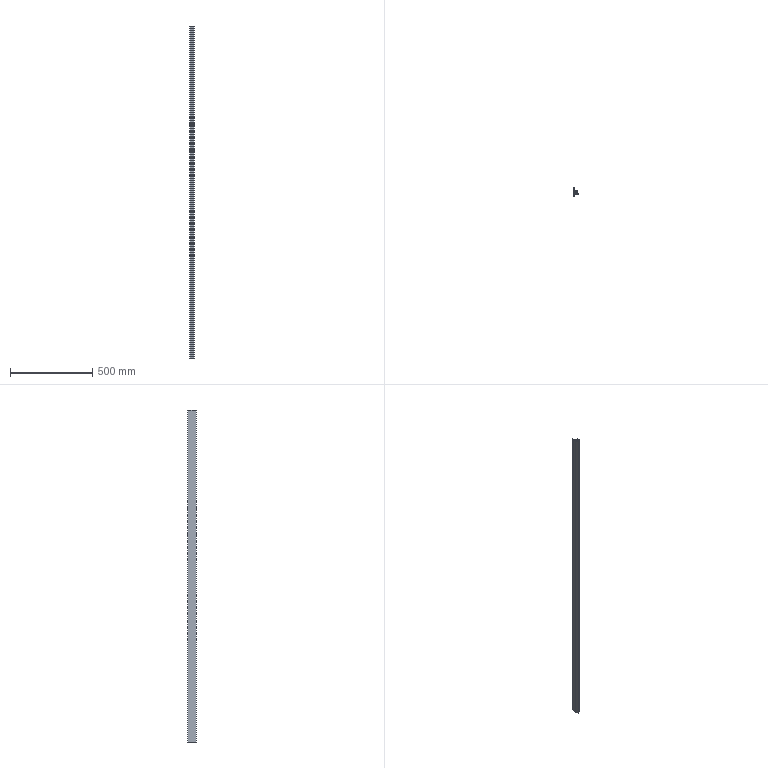Part | 1 solid | 43 faces | box 25 x 50 x 2016 mm | volume 628045 mm3 | plane 35 | cylinder 8 | commonest cylinder face diameters 0.6 x8
STEP:
#1=CARTESIAN_POINT('',(1.5,0.,1008.));
#2=VERTEX_POINT('',#1);
#3=CARTESIAN_POINT('',(1.5,10.,1008.));
#4=VERTEX_POINT('',#3);
#5=CARTESIAN_POINT('',(1.5,0.,1008.));
#6=DIRECTION('',(0.,1.,0.));
#7=VECTOR('',#6,1000.);
#8=LINE('',#5,#7);
#9=EDGE_CURVE('',#2,#4,#8,.T.);
#10=ORIENTED_EDGE('',*,*,#9,.T.);
#11=CARTESIAN_POINT('',(4.,10.,1008.));
#12=VERTEX_POINT('',#11);
#13=CARTESIAN_POINT('',(1.5,10.,1008.));
#14=DIRECTION('',(1.,0.,0.));
#15=VECTOR('',#14,1000.);
#16=LINE('',#13,#15);
#17=EDGE_CURVE('',#4,#12,#16,.T.);
#18=ORIENTED_EDGE('',*,*,#17,.T.);
#19=CARTESIAN_POINT('',(4.,10.5,1008.));
#20=VERTEX_POINT('',#19);
#21=CARTESIAN_POINT('',(4.,10.,1008.));
#22=DIRECTION('',(0.,1.,0.));
#23=VECTOR('',#22,1000.);
#24=LINE('',#21,#23);
#25=EDGE_CURVE('',#12,#20,#24,.T.);
#26=ORIENTED_EDGE('',*,*,#25,.T.);
#27=CARTESIAN_POINT('',(8.9,10.5,1008.));
#28=VERTEX_POINT('',#27);
#29=CARTESIAN_POINT('',(4.,10.5,1008.));
#30=DIRECTION('',(1.,0.,0.));
#31=VECTOR('',#30,1000.);
#32=LINE('',#29,#31);
#33=EDGE_CURVE('',#20,#28,#32,.T.);
#34=ORIENTED_EDGE('',*,*,#33,.T.);
#35=CARTESIAN_POINT('',(8.9,12.2,1008.));
#36=VERTEX_POINT('',#35);
#37=CARTESIAN_POINT('',(8.9,10.5,1008.));
#38=DIRECTION('',(0.,1.,0.));
#39=VECTOR('',#38,1000.);
#40=LINE('',#37,#39);
#41=EDGE_CURVE('',#28,#36,#40,.T.);
#42=ORIENTED_EDGE('',*,*,#41,.T.);
#43=CARTESIAN_POINT('',(8.6,12.5,1008.));
#44=VERTEX_POINT('',#43);
#45=CARTESIAN_POINT('',(8.6,12.2,1008.));
#46=DIRECTION('',(0.,0.,1.));
#47=DIRECTION('',(1.,0.,0.));
#48=AXIS2_PLACEMENT_3D('',#45,#46,#47);
#49=CIRCLE('',#48,0.3);
#50=EDGE_CURVE('',#36,#44,#49,.T.);
#51=ORIENTED_EDGE('',*,*,#50,.T.);
#52=CARTESIAN_POINT('',(5.05,12.5,1008.));
#53=VERTEX_POINT('',#52);
#54=CARTESIAN_POINT('',(8.6,12.5,1008.));
#55=DIRECTION('',(-1.,0.,0.));
#56=VECTOR('',#55,1000.);
#57=LINE('',#54,#56);
#58=EDGE_CURVE('',#44,#53,#57,.T.);
#59=ORIENTED_EDGE('',*,*,#58,.T.);
#60=CARTESIAN_POINT('',(4.75,12.8,1008.));
#61=VERTEX_POINT('',#60);
#62=CARTESIAN_POINT('',(5.05,12.8,1008.));
#63=DIRECTION('',(0.,0.,-1.));
#64=DIRECTION('',(1.,0.,0.));
#65=AXIS2_PLACEMENT_3D('',#62,#63,#64);
#66=CIRCLE('',#65,0.3);
#67=EDGE_CURVE('',#53,#61,#66,.T.);
#68=ORIENTED_EDGE('',*,*,#67,.T.);
#69=CARTESIAN_POINT('',(4.75,16.153,1008.));
#70=VERTEX_POINT('',#69);
#71=CARTESIAN_POINT('',(4.75,12.8,1008.));
#72=DIRECTION('',(0.,1.,0.));
#73=VECTOR('',#72,1000.);
#74=LINE('',#71,#73);
#75=EDGE_CURVE('',#61,#70,#74,.T.);
#76=ORIENTED_EDGE('',*,*,#75,.T.);
#77=CARTESIAN_POINT('',(4.838,16.365,1008.));
#78=VERTEX_POINT('',#77);
#79=CARTESIAN_POINT('',(5.05,16.153,1008.));
#80=DIRECTION('',(0.,0.,-1.));
#81=DIRECTION('',(1.,0.,0.));
#82=AXIS2_PLACEMENT_3D('',#79,#80,#81);
#83=CIRCLE('',#82,0.3);
#84=EDGE_CURVE('',#70,#78,#83,.T.);
#85=ORIENTED_EDGE('',*,*,#84,.T.);
#86=CARTESIAN_POINT('',(8.785,20.312,1008.));
#87=VERTEX_POINT('',#86);
#88=CARTESIAN_POINT('',(4.838,16.365,1008.));
#89=DIRECTION('',(0.7071,0.7071,0.));
#90=VECTOR('',#89,1000.);
#91=LINE('',#88,#90);
#92=EDGE_CURVE('',#78,#87,#91,.T.);
#93=ORIENTED_EDGE('',*,*,#92,.T.);
#94=CARTESIAN_POINT('',(8.997,20.4,1008.));
#95=VERTEX_POINT('',#94);
#96=CARTESIAN_POINT('',(8.997,20.1,1008.));
#97=DIRECTION('',(0.,0.,-1.));
#98=DIRECTION('',(1.,0.,0.));
#99=AXIS2_PLACEMENT_3D('',#96,#97,#98);
#100=CIRCLE('',#99,0.3);
#101=EDGE_CURVE('',#87,#95,#100,.T.);
#102=ORIENTED_EDGE('',*,*,#101,.T.);
#103=CARTESIAN_POINT('',(17.003,20.4,1008.));
#104=VERTEX_POINT('',#103);
#105=CARTESIAN_POINT('',(8.997,20.4,1008.));
#106=DIRECTION('',(1.,0.,0.));
#107=VECTOR('',#106,1000.);
#108=LINE('',#105,#107);
#109=EDGE_CURVE('',#95,#104,#108,.T.);
#110=ORIENTED_EDGE('',*,*,#109,.T.);
#111=CARTESIAN_POINT('',(17.215,20.312,1008.));
#112=VERTEX_POINT('',#111);
#113=CARTESIAN_POINT('',(17.003,20.1,1008.));
#114=DIRECTION('',(0.,0.,-1.));
#115=DIRECTION('',(1.,0.,0.));
#116=AXIS2_PLACEMENT_3D('',#113,#114,#115);
#117=CIRCLE('',#116,0.3);
#118=EDGE_CURVE('',#104,#112,#117,.T.);
#119=ORIENTED_EDGE('',*,*,#118,.T.);
#120=CARTESIAN_POINT('',(21.162,16.365,1008.));
#121=VERTEX_POINT('',#120);
#122=CARTESIAN_POINT('',(17.215,20.312,1008.));
#123=DIRECTION('',(0.7071,-0.7071,0.));
#124=VECTOR('',#123,1000.);
#125=LINE('',#122,#124);
#126=EDGE_CURVE('',#112,#121,#125,.T.);
#127=ORIENTED_EDGE('',*,*,#126,.T.);
#128=CARTESIAN_POINT('',(21.25,16.153,1008.));
#129=VERTEX_POINT('',#128);
#130=CARTESIAN_POINT('',(20.95,16.153,1008.));
#131=DIRECTION('',(0.,0.,-1.));
#132=DIRECTION('',(1.,0.,0.));
#133=AXIS2_PLACEMENT_3D('',#130,#131,#132);
#134=CIRCLE('',#133,0.3);
#135=EDGE_CURVE('',#121,#129,#134,.T.);
#136=ORIENTED_EDGE('',*,*,#135,.T.);
#137=CARTESIAN_POINT('',(21.25,12.8,1008.));
#138=VERTEX_POINT('',#137);
#139=CARTESIAN_POINT('',(21.25,16.153,1008.));
#140=DIRECTION('',(0.,-1.,0.));
#141=VECTOR('',#140,1000.);
#142=LINE('',#139,#141);
#143=EDGE_CURVE('',#129,#138,#142,.T.);
#144=ORIENTED_EDGE('',*,*,#143,.T.);
#145=CARTESIAN_POINT('',(20.95,12.5,1008.));
#146=VERTEX_POINT('',#145);
#147=CARTESIAN_POINT('',(20.95,12.8,1008.));
#148=DIRECTION('',(0.,0.,-1.));
#149=DIRECTION('',(1.,0.,0.));
#150=AXIS2_PLACEMENT_3D('',#147,#148,#149);
#151=CIRCLE('',#150,0.3);
#152=EDGE_CURVE('',#138,#146,#151,.T.);
#153=ORIENTED_EDGE('',*,*,#152,.T.);
#154=CARTESIAN_POINT('',(17.4,12.5,1008.));
#155=VERTEX_POINT('',#154);
#156=CARTESIAN_POINT('',(20.95,12.5,1008.));
#157=DIRECTION('',(-1.,0.,0.));
#158=VECTOR('',#157,1000.);
#159=LINE('',#156,#158);
#160=EDGE_CURVE('',#146,#155,#159,.T.);
#161=ORIENTED_EDGE('',*,*,#160,.T.);
#162=CARTESIAN_POINT('',(17.1,12.2,1008.));
#163=VERTEX_POINT('',#162);
#164=CARTESIAN_POINT('',(17.4,12.2,1008.));
#165=DIRECTION('',(0.,0.,1.));
#166=DIRECTION('',(1.,0.,0.));
#167=AXIS2_PLACEMENT_3D('',#164,#165,#166);
#168=CIRCLE('',#167,0.3);
#169=EDGE_CURVE('',#155,#163,#168,.T.);
#170=ORIENTED_EDGE('',*,*,#169,.T.);
#171=CARTESIAN_POINT('',(17.1,10.5,1008.));
#172=VERTEX_POINT('',#171);
#173=CARTESIAN_POINT('',(17.1,12.2,1008.));
#174=DIRECTION('',(0.,-1.,0.));
#175=VECTOR('',#174,1000.);
#176=LINE('',#173,#175);
#177=EDGE_CURVE('',#163,#172,#176,.T.);
#178=ORIENTED_EDGE('',*,*,#177,.T.);
#179=CARTESIAN_POINT('',(22.,10.5,1008.));
#180=VERTEX_POINT('',#179);
#181=CARTESIAN_POINT('',(17.1,10.5,1008.));
#182=DIRECTION('',(1.,0.,0.));
#183=VECTOR('',#182,1000.);
#184=LINE('',#181,#183);
#185=EDGE_CURVE('',#172,#180,#184,.T.);
#186=ORIENTED_EDGE('',*,*,#185,.T.);
#187=CARTESIAN_POINT('',(22.,10.,1008.));
#188=VERTEX_POINT('',#187);
#189=CARTESIAN_POINT('',(22.,10.5,1008.));
#190=DIRECTION('',(0.,-1.,0.));
#191=VECTOR('',#190,1000.);
#192=LINE('',#189,#191);
#193=EDGE_CURVE('',#180,#188,#192,.T.);
#194=ORIENTED_EDGE('',*,*,#193,.T.);
#195=CARTESIAN_POINT('',(25.,10.,1008.));
#196=VERTEX_POINT('',#195);
#197=CARTESIAN_POINT('',(22.,10.,1008.));
#198=DIRECTION('',(1.,0.,0.));
#199=VECTOR('',#198,1000.);
#200=LINE('',#197,#199);
#201=EDGE_CURVE('',#188,#196,#200,.T.);
#202=ORIENTED_EDGE('',*,*,#201,.T.);
#203=CARTESIAN_POINT('',(25.,15.,1008.));
#204=VERTEX_POINT('',#203);
#205=CARTESIAN_POINT('',(25.,10.,1008.));
#206=DIRECTION('',(0.,1.,0.));
#207=VECTOR('',#206,1000.);
#208=LINE('',#205,#207);
#209=EDGE_CURVE('',#196,#204,#208,.T.);
#210=ORIENTED_EDGE('',*,*,#209,.T.);
#211=CARTESIAN_POINT('',(23.,15.,1008.));
#212=VERTEX_POINT('',#211);
#213=CARTESIAN_POINT('',(25.,15.,1008.));
#214=DIRECTION('',(-1.,0.,0.));
#215=VECTOR('',#214,1000.);
#216=LINE('',#213,#215);
#217=EDGE_CURVE('',#204,#212,#216,.T.);
#218=ORIENTED_EDGE('',*,*,#217,.T.);
#219=CARTESIAN_POINT('',(23.,29.246,1008.));
#220=VERTEX_POINT('',#219);
#221=CARTESIAN_POINT('',(23.,15.,1008.));
#222=DIRECTION('',(0.,1.,0.));
#223=VECTOR('',#222,1000.);
#224=LINE('',#221,#223);
#225=EDGE_CURVE('',#212,#220,#224,.T.);
#226=ORIENTED_EDGE('',*,*,#225,.T.);
#227=CARTESIAN_POINT('',(22.25,29.996,1008.));
#228=VERTEX_POINT('',#227);
#229=CARTESIAN_POINT('',(23.,29.246,1008.));
#230=DIRECTION('',(-0.7071,0.7071,0.));
#231=VECTOR('',#230,1000.);
#232=LINE('',#229,#231);
#233=EDGE_CURVE('',#220,#228,#232,.T.);
#234=ORIENTED_EDGE('',*,*,#233,.T.);
#235=CARTESIAN_POINT('',(4.,30.,1008.));
#236=VERTEX_POINT('',#235);
#237=CARTESIAN_POINT('',(22.25,29.996,1008.));
#238=DIRECTION('',(-1.,0.0002341,0.));
#239=VECTOR('',#238,1000.);
#240=LINE('',#237,#239);
#241=EDGE_CURVE('',#228,#236,#240,.T.);
#242=ORIENTED_EDGE('',*,*,#241,.T.);
#243=CARTESIAN_POINT('',(4.,34.998,1008.));
#244=VERTEX_POINT('',#243);
#245=CARTESIAN_POINT('',(4.,30.,1008.));
#246=DIRECTION('',(0.,1.,0.));
#247=VECTOR('',#246,1000.);
#248=LINE('',#245,#247);
#249=EDGE_CURVE('',#236,#244,#248,.T.);
#250=ORIENTED_EDGE('',*,*,#249,.T.);
#251=CARTESIAN_POINT('',(3.,34.998,1008.));
#252=VERTEX_POINT('',#251);
#253=CARTESIAN_POINT('',(4.,34.998,1008.));
#254=DIRECTION('',(-1.,0.,0.));
#255=VECTOR('',#254,1000.);
#256=LINE('',#253,#255);
#257=EDGE_CURVE('',#244,#252,#256,.T.);
#258=ORIENTED_EDGE('',*,*,#257,.T.);
#259=CARTESIAN_POINT('',(3.,43.,1008.));
#260=VERTEX_POINT('',#259);
#261=CARTESIAN_POINT('',(3.,34.998,1008.));
#262=DIRECTION('',(0.,1.,0.));
#263=VECTOR('',#262,1000.);
#264=LINE('',#261,#263);
#265=EDGE_CURVE('',#252,#260,#264,.T.);
#266=ORIENTED_EDGE('',*,*,#265,.T.);
#267=CARTESIAN_POINT('',(4.,43.,1008.));
#268=VERTEX_POINT('',#267);
#269=CARTESIAN_POINT('',(3.,43.,1008.));
#270=DIRECTION('',(1.,0.,0.));
#271=VECTOR('',#270,1000.);
#272=LINE('',#269,#271);
#273=EDGE_CURVE('',#260,#268,#272,.T.);
#274=ORIENTED_EDGE('',*,*,#273,.T.);
#275=CARTESIAN_POINT('',(4.,50.,1008.));
#276=VERTEX_POINT('',#275);
#277=CARTESIAN_POINT('',(4.,43.,1008.));
#278=DIRECTION('',(0.,1.,0.));
#279=VECTOR('',#278,1000.);
#280=LINE('',#277,#279);
#281=EDGE_CURVE('',#268,#276,#280,.T.);
#282=ORIENTED_EDGE('',*,*,#281,.T.);
#283=CARTESIAN_POINT('',(0.,50.,1008.));
#284=VERTEX_POINT('',#283);
#285=CARTESIAN_POINT('',(4.,50.,1008.));
#286=DIRECTION('',(-1.,0.,0.));
#287=VECTOR('',#286,1000.);
#288=LINE('',#285,#287);
#289=EDGE_CURVE('',#276,#284,#288,.T.);
#290=ORIENTED_EDGE('',*,*,#289,.T.);
#291=CARTESIAN_POINT('',(0.,0.,1008.));
#292=VERTEX_POINT('',#291);
#293=CARTESIAN_POINT('',(0.,50.,1008.));
#294=DIRECTION('',(0.,-1.,0.));
#295=VECTOR('',#294,1000.);
#296=LINE('',#293,#295);
#297=EDGE_CURVE('',#284,#292,#296,.T.);
#298=ORIENTED_EDGE('',*,*,#297,.T.);
#299=CARTESIAN_POINT('',(0.,0.,1008.));
#300=DIRECTION('',(1.,0.,0.));
#301=VECTOR('',#300,1000.);
#302=LINE('',#299,#301);
#303=EDGE_CURVE('',#292,#2,#302,.T.);
#304=ORIENTED_EDGE('',*,*,#303,.T.);
#305=EDGE_LOOP('',(#10,#18,#26,#34,#42,#51,#59,#68,#76,#85,#93,#102,#110,#119,#127,#136,#144,#153,#161,#170,#178,#186,#194,#202,#210,#218,#226,#234,#242,#250,#258,#266,#274,#282,#290,#298,#304));
#306=FACE_OUTER_BOUND('',#305,.T.);
#307=CARTESIAN_POINT('',(21.,28.,1008.));
#308=VERTEX_POINT('',#307);
#309=CARTESIAN_POINT('',(2.,28.,1008.));
#310=VERTEX_POINT('',#309);
#311=CARTESIAN_POINT('',(2.,28.,1008.));
#312=DIRECTION('',(-1.,0.,0.));
#313=VECTOR('',#312,1000.);
#314=LINE('',#311,#313);
#315=EDGE_CURVE('',#308,#310,#314,.T.);
#316=ORIENTED_EDGE('',*,*,#315,.F.);
#317=CARTESIAN_POINT('',(21.,22.4,1008.));
#318=VERTEX_POINT('',#317);
#319=CARTESIAN_POINT('',(21.,28.,1008.));
#320=DIRECTION('',(0.,1.,0.));
#321=VECTOR('',#320,1000.);
#322=LINE('',#319,#321);
#323=EDGE_CURVE('',#318,#308,#322,.T.);
#324=ORIENTED_EDGE('',*,*,#323,.F.);
#325=CARTESIAN_POINT('',(2.,22.4,1008.));
#326=VERTEX_POINT('',#325);
#327=CARTESIAN_POINT('',(21.,22.4,1008.));
#328=DIRECTION('',(1.,0.,0.));
#329=VECTOR('',#328,1000.);
#330=LINE('',#327,#329);
#331=EDGE_CURVE('',#326,#318,#330,.T.);
#332=ORIENTED_EDGE('',*,*,#331,.F.);
#333=CARTESIAN_POINT('',(2.,22.4,1008.));
#334=DIRECTION('',(0.,-1.,0.));
#335=VECTOR('',#334,1000.);
#336=LINE('',#333,#335);
#337=EDGE_CURVE('',#310,#326,#336,.T.);
#338=ORIENTED_EDGE('',*,*,#337,.F.);
#339=EDGE_LOOP('',(#316,#324,#332,#338));
#340=FACE_BOUND('',#339,.T.);
#341=CARTESIAN_POINT('',(8.6,12.2,1008.));
#342=DIRECTION('',(0.,0.,1.));
#343=DIRECTION('',(1.,0.,0.));
#344=AXIS2_PLACEMENT_3D('',#341,#342,#343);
#345=PLANE('',#344);
#346=ADVANCED_FACE('',(#306,#340),#345,.T.);
#347=CARTESIAN_POINT('',(1.5,0.,-1008.));
#348=VERTEX_POINT('',#347);
#349=CARTESIAN_POINT('',(1.5,10.,-1008.));
#350=VERTEX_POINT('',#349);
#351=CARTESIAN_POINT('',(1.5,0.,-1008.));
#352=DIRECTION('',(0.,1.,0.));
#353=VECTOR('',#352,1000.);
#354=LINE('',#351,#353);
#355=EDGE_CURVE('',#348,#350,#354,.T.);
#356=ORIENTED_EDGE('',*,*,#355,.F.);
#357=CARTESIAN_POINT('',(0.,0.,-1008.));
#358=VERTEX_POINT('',#357);
#359=CARTESIAN_POINT('',(0.,0.,-1008.));
#360=DIRECTION('',(1.,0.,0.));
#361=VECTOR('',#360,1000.);
#362=LINE('',#359,#361);
#363=EDGE_CURVE('',#358,#348,#362,.T.);
#364=ORIENTED_EDGE('',*,*,#363,.F.);
#365=CARTESIAN_POINT('',(0.,50.,-1008.));
#366=VERTEX_POINT('',#365);
#367=CARTESIAN_POINT('',(0.,50.,-1008.));
#368=DIRECTION('',(0.,-1.,0.));
#369=VECTOR('',#368,1000.);
#370=LINE('',#367,#369);
#371=EDGE_CURVE('',#366,#358,#370,.T.);
#372=ORIENTED_EDGE('',*,*,#371,.F.);
#373=CARTESIAN_POINT('',(4.,50.,-1008.));
#374=VERTEX_POINT('',#373);
#375=CARTESIAN_POINT('',(4.,50.,-1008.));
#376=DIRECTION('',(-1.,0.,0.));
#377=VECTOR('',#376,1000.);
#378=LINE('',#375,#377);
#379=EDGE_CURVE('',#374,#366,#378,.T.);
#380=ORIENTED_EDGE('',*,*,#379,.F.);
#381=CARTESIAN_POINT('',(4.,43.,-1008.));
#382=VERTEX_POINT('',#381);
#383=CARTESIAN_POINT('',(4.,43.,-1008.));
#384=DIRECTION('',(0.,1.,0.));
#385=VECTOR('',#384,1000.);
#386=LINE('',#383,#385);
#387=EDGE_CURVE('',#382,#374,#386,.T.);
#388=ORIENTED_EDGE('',*,*,#387,.F.);
#389=CARTESIAN_POINT('',(3.,43.,-1008.));
#390=VERTEX_POINT('',#389);
#391=CARTESIAN_POINT('',(3.,43.,-1008.));
#392=DIRECTION('',(1.,0.,0.));
#393=VECTOR('',#392,1000.);
#394=LINE('',#391,#393);
#395=EDGE_CURVE('',#390,#382,#394,.T.);
#396=ORIENTED_EDGE('',*,*,#395,.F.);
#397=CARTESIAN_POINT('',(3.,34.998,-1008.));
#398=VERTEX_POINT('',#397);
#399=CARTESIAN_POINT('',(3.,34.998,-1008.));
#400=DIRECTION('',(0.,1.,0.));
#401=VECTOR('',#400,1000.);
#402=LINE('',#399,#401);
#403=EDGE_CURVE('',#398,#390,#402,.T.);
#404=ORIENTED_EDGE('',*,*,#403,.F.);
#405=CARTESIAN_POINT('',(4.,34.998,-1008.));
#406=VERTEX_POINT('',#405);
#407=CARTESIAN_POINT('',(4.,34.998,-1008.));
#408=DIRECTION('',(-1.,0.,0.));
#409=VECTOR('',#408,1000.);
#410=LINE('',#407,#409);
#411=EDGE_CURVE('',#406,#398,#410,.T.);
#412=ORIENTED_EDGE('',*,*,#411,.F.);
#413=CARTESIAN_POINT('',(4.,30.,-1008.));
#414=VERTEX_POINT('',#413);
#415=CARTESIAN_POINT('',(4.,30.,-1008.));
#416=DIRECTION('',(0.,1.,0.));
#417=VECTOR('',#416,1000.);
#418=LINE('',#415,#417);
#419=EDGE_CURVE('',#414,#406,#418,.T.);
#420=ORIENTED_EDGE('',*,*,#419,.F.);
#421=CARTESIAN_POINT('',(22.25,29.996,-1008.));
#422=VERTEX_POINT('',#421);
#423=CARTESIAN_POINT('',(22.25,29.996,-1008.));
#424=DIRECTION('',(-1.,0.0002341,0.));
#425=VECTOR('',#424,1000.);
#426=LINE('',#423,#425);
#427=EDGE_CURVE('',#422,#414,#426,.T.);
#428=ORIENTED_EDGE('',*,*,#427,.F.);
#429=CARTESIAN_POINT('',(23.,29.246,-1008.));
#430=VERTEX_POINT('',#429);
#431=CARTESIAN_POINT('',(23.,29.246,-1008.));
#432=DIRECTION('',(-0.7071,0.7071,0.));
#433=VECTOR('',#432,1000.);
#434=LINE('',#431,#433);
#435=EDGE_CURVE('',#430,#422,#434,.T.);
#436=ORIENTED_EDGE('',*,*,#435,.F.);
#437=CARTESIAN_POINT('',(23.,15.,-1008.));
#438=VERTEX_POINT('',#437);
#439=CARTESIAN_POINT('',(23.,15.,-1008.));
#440=DIRECTION('',(0.,1.,0.));
#441=VECTOR('',#440,1000.);
#442=LINE('',#439,#441);
#443=EDGE_CURVE('',#438,#430,#442,.T.);
#444=ORIENTED_EDGE('',*,*,#443,.F.);
#445=CARTESIAN_POINT('',(25.,15.,-1008.));
#446=VERTEX_POINT('',#445);
#447=CARTESIAN_POINT('',(25.,15.,-1008.));
#448=DIRECTION('',(-1.,0.,0.));
#449=VECTOR('',#448,1000.);
#450=LINE('',#447,#449);
#451=EDGE_CURVE('',#446,#438,#450,.T.);
#452=ORIENTED_EDGE('',*,*,#451,.F.);
#453=CARTESIAN_POINT('',(25.,10.,-1008.));
#454=VERTEX_POINT('',#453);
#455=CARTESIAN_POINT('',(25.,10.,-1008.));
#456=DIRECTION('',(0.,1.,0.));
#457=VECTOR('',#456,1000.);
#458=LINE('',#455,#457);
#459=EDGE_CURVE('',#454,#446,#458,.T.);
#460=ORIENTED_EDGE('',*,*,#459,.F.);
#461=CARTESIAN_POINT('',(22.,10.,-1008.));
#462=VERTEX_POINT('',#461);
#463=CARTESIAN_POINT('',(22.,10.,-1008.));
#464=DIRECTION('',(1.,0.,0.));
#465=VECTOR('',#464,1000.);
#466=LINE('',#463,#465);
#467=EDGE_CURVE('',#462,#454,#466,.T.);
#468=ORIENTED_EDGE('',*,*,#467,.F.);
#469=CARTESIAN_POINT('',(22.,10.5,-1008.));
#470=VERTEX_POINT('',#469);
#471=CARTESIAN_POINT('',(22.,10.5,-1008.));
#472=DIRECTION('',(0.,-1.,0.));
#473=VECTOR('',#472,1000.);
#474=LINE('',#471,#473);
#475=EDGE_CURVE('',#470,#462,#474,.T.);
#476=ORIENTED_EDGE('',*,*,#475,.F.);
#477=CARTESIAN_POINT('',(17.1,10.5,-1008.));
#478=VERTEX_POINT('',#477);
#479=CARTESIAN_POINT('',(17.1,10.5,-1008.));
#480=DIRECTION('',(1.,0.,0.));
#481=VECTOR('',#480,1000.);
#482=LINE('',#479,#481);
#483=EDGE_CURVE('',#478,#470,#482,.T.);
#484=ORIENTED_EDGE('',*,*,#483,.F.);
#485=CARTESIAN_POINT('',(17.1,12.2,-1008.));
#486=VERTEX_POINT('',#485);
#487=CARTESIAN_POINT('',(17.1,12.2,-1008.));
#488=DIRECTION('',(0.,-1.,0.));
#489=VECTOR('',#488,1000.);
#490=LINE('',#487,#489);
#491=EDGE_CURVE('',#486,#478,#490,.T.);
#492=ORIENTED_EDGE('',*,*,#491,.F.);
#493=CARTESIAN_POINT('',(17.4,12.5,-1008.));
#494=VERTEX_POINT('',#493);
#495=CARTESIAN_POINT('',(17.4,12.2,-1008.));
#496=DIRECTION('',(0.,0.,1.));
#497=DIRECTION('',(1.,0.,0.));
#498=AXIS2_PLACEMENT_3D('',#495,#496,#497);
#499=CIRCLE('',#498,0.3);
#500=EDGE_CURVE('',#494,#486,#499,.T.);
#501=ORIENTED_EDGE('',*,*,#500,.F.);
#502=CARTESIAN_POINT('',(20.95,12.5,-1008.));
#503=VERTEX_POINT('',#502);
#504=CARTESIAN_POINT('',(20.95,12.5,-1008.));
#505=DIRECTION('',(-1.,0.,0.));
#506=VECTOR('',#505,1000.);
#507=LINE('',#504,#506);
#508=EDGE_CURVE('',#503,#494,#507,.T.);
#509=ORIENTED_EDGE('',*,*,#508,.F.);
#510=CARTESIAN_POINT('',(21.25,12.8,-1008.));
#511=VERTEX_POINT('',#510);
#512=CARTESIAN_POINT('',(20.95,12.8,-1008.));
#513=DIRECTION('',(0.,0.,-1.));
#514=DIRECTION('',(1.,0.,0.));
#515=AXIS2_PLACEMENT_3D('',#512,#513,#514);
#516=CIRCLE('',#515,0.3);
#517=EDGE_CURVE('',#511,#503,#516,.T.);
#518=ORIENTED_EDGE('',*,*,#517,.F.);
#519=CARTESIAN_POINT('',(21.25,16.153,-1008.));
#520=VERTEX_POINT('',#519);
#521=CARTESIAN_POINT('',(21.25,16.153,-1008.));
#522=DIRECTION('',(0.,-1.,0.));
#523=VECTOR('',#522,1000.);
#524=LINE('',#521,#523);
#525=EDGE_CURVE('',#520,#511,#524,.T.);
#526=ORIENTED_EDGE('',*,*,#525,.F.);
#527=CARTESIAN_POINT('',(21.162,16.365,-1008.));
#528=VERTEX_POINT('',#527);
#529=CARTESIAN_POINT('',(20.95,16.153,-1008.));
#530=DIRECTION('',(0.,0.,-1.));
#531=DIRECTION('',(1.,0.,0.));
#532=AXIS2_PLACEMENT_3D('',#529,#530,#531);
#533=CIRCLE('',#532,0.3);
#534=EDGE_CURVE('',#528,#520,#533,.T.);
#535=ORIENTED_EDGE('',*,*,#534,.F.);
#536=CARTESIAN_POINT('',(17.215,20.312,-1008.));
#537=VERTEX_POINT('',#536);
#538=CARTESIAN_POINT('',(17.215,20.312,-1008.));
#539=DIRECTION('',(0.7071,-0.7071,0.));
#540=VECTOR('',#539,1000.);
#541=LINE('',#538,#540);
#542=EDGE_CURVE('',#537,#528,#541,.T.);
#543=ORIENTED_EDGE('',*,*,#542,.F.);
#544=CARTESIAN_POINT('',(17.003,20.4,-1008.));
#545=VERTEX_POINT('',#544);
#546=CARTESIAN_POINT('',(17.003,20.1,-1008.));
#547=DIRECTION('',(0.,0.,-1.));
#548=DIRECTION('',(1.,0.,0.));
#549=AXIS2_PLACEMENT_3D('',#546,#547,#548);
#550=CIRCLE('',#549,0.3);
#551=EDGE_CURVE('',#545,#537,#550,.T.);
#552=ORIENTED_EDGE('',*,*,#551,.F.);
#553=CARTESIAN_POINT('',(8.997,20.4,-1008.));
#554=VERTEX_POINT('',#553);
#555=CARTESIAN_POINT('',(8.997,20.4,-1008.));
#556=DIRECTION('',(1.,0.,0.));
#557=VECTOR('',#556,1000.);
#558=LINE('',#555,#557);
#559=EDGE_CURVE('',#554,#545,#558,.T.);
#560=ORIENTED_EDGE('',*,*,#559,.F.);
#561=CARTESIAN_POINT('',(8.785,20.312,-1008.));
#562=VERTEX_POINT('',#561);
#563=CARTESIAN_POINT('',(8.997,20.1,-1008.));
#564=DIRECTION('',(0.,0.,-1.));
#565=DIRECTION('',(1.,0.,0.));
#566=AXIS2_PLACEMENT_3D('',#563,#564,#565);
#567=CIRCLE('',#566,0.3);
#568=EDGE_CURVE('',#562,#554,#567,.T.);
#569=ORIENTED_EDGE('',*,*,#568,.F.);
#570=CARTESIAN_POINT('',(4.838,16.365,-1008.));
#571=VERTEX_POINT('',#570);
#572=CARTESIAN_POINT('',(4.838,16.365,-1008.));
#573=DIRECTION('',(0.7071,0.7071,0.));
#574=VECTOR('',#573,1000.);
#575=LINE('',#572,#574);
#576=EDGE_CURVE('',#571,#562,#575,.T.);
#577=ORIENTED_EDGE('',*,*,#576,.F.);
#578=CARTESIAN_POINT('',(4.75,16.153,-1008.));
#579=VERTEX_POINT('',#578);
#580=CARTESIAN_POINT('',(5.05,16.153,-1008.));
#581=DIRECTION('',(0.,0.,-1.));
#582=DIRECTION('',(1.,0.,0.));
#583=AXIS2_PLACEMENT_3D('',#580,#581,#582);
#584=CIRCLE('',#583,0.3);
#585=EDGE_CURVE('',#579,#571,#584,.T.);
#586=ORIENTED_EDGE('',*,*,#585,.F.);
#587=CARTESIAN_POINT('',(4.75,12.8,-1008.));
#588=VERTEX_POINT('',#587);
#589=CARTESIAN_POINT('',(4.75,12.8,-1008.));
#590=DIRECTION('',(0.,1.,0.));
#591=VECTOR('',#590,1000.);
#592=LINE('',#589,#591);
#593=EDGE_CURVE('',#588,#579,#592,.T.);
#594=ORIENTED_EDGE('',*,*,#593,.F.);
#595=CARTESIAN_POINT('',(5.05,12.5,-1008.));
#596=VERTEX_POINT('',#595);
#597=CARTESIAN_POINT('',(5.05,12.8,-1008.));
#598=DIRECTION('',(0.,0.,-1.));
#599=DIRECTION('',(1.,0.,0.));
#600=AXIS2_PLACEMENT_3D('',#597,#598,#599);
#601=CIRCLE('',#600,0.3);
#602=EDGE_CURVE('',#596,#588,#601,.T.);
#603=ORIENTED_EDGE('',*,*,#602,.F.);
#604=CARTESIAN_POINT('',(8.6,12.5,-1008.));
#605=VERTEX_POINT('',#604);
#606=CARTESIAN_POINT('',(8.6,12.5,-1008.));
#607=DIRECTION('',(-1.,0.,0.));
#608=VECTOR('',#607,1000.);
#609=LINE('',#606,#608);
#610=EDGE_CURVE('',#605,#596,#609,.T.);
#611=ORIENTED_EDGE('',*,*,#610,.F.);
#612=CARTESIAN_POINT('',(8.9,12.2,-1008.));
#613=VERTEX_POINT('',#612);
#614=CARTESIAN_POINT('',(8.6,12.2,-1008.));
#615=DIRECTION('',(0.,0.,1.));
#616=DIRECTION('',(1.,0.,0.));
#617=AXIS2_PLACEMENT_3D('',#614,#615,#616);
#618=CIRCLE('',#617,0.3);
#619=EDGE_CURVE('',#613,#605,#618,.T.);
#620=ORIENTED_EDGE('',*,*,#619,.F.);
#621=CARTESIAN_POINT('',(8.9,10.5,-1008.));
#622=VERTEX_POINT('',#621);
#623=CARTESIAN_POINT('',(8.9,10.5,-1008.));
#624=DIRECTION('',(0.,1.,0.));
#625=VECTOR('',#624,1000.);
#626=LINE('',#623,#625);
#627=EDGE_CURVE('',#622,#613,#626,.T.);
#628=ORIENTED_EDGE('',*,*,#627,.F.);
#629=CARTESIAN_POINT('',(4.,10.5,-1008.));
#630=VERTEX_POINT('',#629);
#631=CARTESIAN_POINT('',(4.,10.5,-1008.));
#632=DIRECTION('',(1.,0.,0.));
#633=VECTOR('',#632,1000.);
#634=LINE('',#631,#633);
#635=EDGE_CURVE('',#630,#622,#634,.T.);
#636=ORIENTED_EDGE('',*,*,#635,.F.);
#637=CARTESIAN_POINT('',(4.,10.,-1008.));
#638=VERTEX_POINT('',#637);
#639=CARTESIAN_POINT('',(4.,10.,-1008.));
#640=DIRECTION('',(0.,1.,0.));
#641=VECTOR('',#640,1000.);
#642=LINE('',#639,#641);
#643=EDGE_CURVE('',#638,#630,#642,.T.);
#644=ORIENTED_EDGE('',*,*,#643,.F.);
#645=CARTESIAN_POINT('',(1.5,10.,-1008.));
#646=DIRECTION('',(1.,0.,0.));
#647=VECTOR('',#646,1000.);
#648=LINE('',#645,#647);
#649=EDGE_CURVE('',#350,#638,#648,.T.);
#650=ORIENTED_EDGE('',*,*,#649,.F.);
#651=EDGE_LOOP('',(#356,#364,#372,#380,#388,#396,#404,#412,#420,#428,#436,#444,#452,#460,#468,#476,#484,#492,#501,#509,#518,#526,#535,#543,#552,#560,#569,#577,#586,#594,#603,#611,#620,#628,#636,#644,#650));
#652=FACE_OUTER_BOUND('',#651,.T.);
#653=CARTESIAN_POINT('',(21.,22.4,-1008.));
#654=VERTEX_POINT('',#653);
#655=CARTESIAN_POINT('',(21.,28.,-1008.));
#656=VERTEX_POINT('',#655);
#657=CARTESIAN_POINT('',(21.,28.,-1008.));
#658=DIRECTION('',(0.,1.,0.));
#659=VECTOR('',#658,1000.);
#660=LINE('',#657,#659);
#661=EDGE_CURVE('',#654,#656,#660,.T.);
#662=ORIENTED_EDGE('',*,*,#661,.T.);
#663=CARTESIAN_POINT('',(2.,28.,-1008.));
#664=VERTEX_POINT('',#663);
#665=CARTESIAN_POINT('',(2.,28.,-1008.));
#666=DIRECTION('',(-1.,0.,0.));
#667=VECTOR('',#666,1000.);
#668=LINE('',#665,#667);
#669=EDGE_CURVE('',#656,#664,#668,.T.);
#670=ORIENTED_EDGE('',*,*,#669,.T.);
#671=CARTESIAN_POINT('',(2.,22.4,-1008.));
#672=VERTEX_POINT('',#671);
#673=CARTESIAN_POINT('',(2.,22.4,-1008.));
#674=DIRECTION('',(0.,-1.,0.));
#675=VECTOR('',#674,1000.);
#676=LINE('',#673,#675);
#677=EDGE_CURVE('',#664,#672,#676,.T.);
#678=ORIENTED_EDGE('',*,*,#677,.T.);
#679=CARTESIAN_POINT('',(21.,22.4,-1008.));
#680=DIRECTION('',(1.,0.,0.));
#681=VECTOR('',#680,1000.);
#682=LINE('',#679,#681);
#683=EDGE_CURVE('',#672,#654,#682,.T.);
#684=ORIENTED_EDGE('',*,*,#683,.T.);
#685=EDGE_LOOP('',(#662,#670,#678,#684));
#686=FACE_BOUND('',#685,.T.);
#687=CARTESIAN_POINT('',(8.6,12.2,-1008.));
#688=DIRECTION('',(0.,0.,1.));
#689=DIRECTION('',(1.,0.,0.));
#690=AXIS2_PLACEMENT_3D('',#687,#688,#689);
#691=PLANE('',#690);
#692=ADVANCED_FACE('',(#652,#686),#691,.F.);
#693=ORIENTED_EDGE('',*,*,#355,.T.);
#694=CARTESIAN_POINT('',(1.5,10.,1008.));
#695=DIRECTION('',(0.,0.,-1.));
#696=VECTOR('',#695,1000.);
#697=LINE('',#694,#696);
#698=EDGE_CURVE('',#4,#350,#697,.T.);
#699=ORIENTED_EDGE('',*,*,#698,.F.);
#700=ORIENTED_EDGE('',*,*,#9,.F.);
#701=CARTESIAN_POINT('',(1.5,0.,1008.));
#702=DIRECTION('',(0.,0.,-1.));
#703=VECTOR('',#702,1000.);
#704=LINE('',#701,#703);
#705=EDGE_CURVE('',#2,#348,#704,.T.);
#706=ORIENTED_EDGE('',*,*,#705,.T.);
#707=EDGE_LOOP('',(#693,#699,#700,#706));
#708=FACE_OUTER_BOUND('',#707,.T.);
#709=CARTESIAN_POINT('',(1.5,0.,1008.));
#710=DIRECTION('',(-1.,0.,0.));
#711=DIRECTION('',(0.,0.,1.));
#712=AXIS2_PLACEMENT_3D('',#709,#710,#711);
#713=PLANE('',#712);
#714=ADVANCED_FACE('',(#708),#713,.F.);
#715=ORIENTED_EDGE('',*,*,#649,.T.);
#716=CARTESIAN_POINT('',(4.,10.,1008.));
#717=DIRECTION('',(0.,0.,-1.));
#718=VECTOR('',#717,1000.);
#719=LINE('',#716,#718);
#720=EDGE_CURVE('',#12,#638,#719,.T.);
#721=ORIENTED_EDGE('',*,*,#720,.F.);
#722=ORIENTED_EDGE('',*,*,#17,.F.);
#723=ORIENTED_EDGE('',*,*,#698,.T.);
#724=EDGE_LOOP('',(#715,#721,#722,#723));
#725=FACE_OUTER_BOUND('',#724,.T.);
#726=CARTESIAN_POINT('',(1.5,10.,1008.));
#727=DIRECTION('',(0.,1.,0.));
#728=DIRECTION('',(0.,0.,1.));
#729=AXIS2_PLACEMENT_3D('',#726,#727,#728);
#730=PLANE('',#729);
#731=ADVANCED_FACE('',(#725),#730,.F.);
#732=ORIENTED_EDGE('',*,*,#643,.T.);
#733=CARTESIAN_POINT('',(4.,10.5,1008.));
#734=DIRECTION('',(0.,0.,-1.));
#735=VECTOR('',#734,1000.);
#736=LINE('',#733,#735);
#737=EDGE_CURVE('',#20,#630,#736,.T.);
#738=ORIENTED_EDGE('',*,*,#737,.F.);
#739=ORIENTED_EDGE('',*,*,#25,.F.);
#740=ORIENTED_EDGE('',*,*,#720,.T.);
#741=EDGE_LOOP('',(#732,#738,#739,#740));
#742=FACE_OUTER_BOUND('',#741,.T.);
#743=CARTESIAN_POINT('',(4.,10.,1008.));
#744=DIRECTION('',(-1.,0.,0.));
#745=DIRECTION('',(0.,0.,1.));
#746=AXIS2_PLACEMENT_3D('',#743,#744,#745);
#747=PLANE('',#746);
#748=ADVANCED_FACE('',(#742),#747,.F.);
#749=ORIENTED_EDGE('',*,*,#635,.T.);
#750=CARTESIAN_POINT('',(8.9,10.5,1008.));
#751=DIRECTION('',(0.,0.,-1.));
#752=VECTOR('',#751,1000.);
#753=LINE('',#750,#752);
#754=EDGE_CURVE('',#28,#622,#753,.T.);
#755=ORIENTED_EDGE('',*,*,#754,.F.);
#756=ORIENTED_EDGE('',*,*,#33,.F.);
#757=ORIENTED_EDGE('',*,*,#737,.T.);
#758=EDGE_LOOP('',(#749,#755,#756,#757));
#759=FACE_OUTER_BOUND('',#758,.T.);
#760=CARTESIAN_POINT('',(4.,10.5,1008.));
#761=DIRECTION('',(0.,1.,0.));
#762=DIRECTION('',(0.,0.,1.));
#763=AXIS2_PLACEMENT_3D('',#760,#761,#762);
#764=PLANE('',#763);
#765=ADVANCED_FACE('',(#759),#764,.F.);
#766=ORIENTED_EDGE('',*,*,#627,.T.);
#767=CARTESIAN_POINT('',(8.9,12.2,1008.));
#768=DIRECTION('',(0.,0.,-1.));
#769=VECTOR('',#768,1000.);
#770=LINE('',#767,#769);
#771=EDGE_CURVE('',#36,#613,#770,.T.);
#772=ORIENTED_EDGE('',*,*,#771,.F.);
#773=ORIENTED_EDGE('',*,*,#41,.F.);
#774=ORIENTED_EDGE('',*,*,#754,.T.);
#775=EDGE_LOOP('',(#766,#772,#773,#774));
#776=FACE_OUTER_BOUND('',#775,.T.);
#777=CARTESIAN_POINT('',(8.9,10.5,1008.));
#778=DIRECTION('',(-1.,0.,0.));
#779=DIRECTION('',(0.,0.,1.));
#780=AXIS2_PLACEMENT_3D('',#777,#778,#779);
#781=PLANE('',#780);
#782=ADVANCED_FACE('',(#776),#781,.F.);
#783=ORIENTED_EDGE('',*,*,#619,.T.);
#784=CARTESIAN_POINT('',(8.6,12.5,1008.));
#785=DIRECTION('',(0.,0.,-1.));
#786=VECTOR('',#785,1000.);
#787=LINE('',#784,#786);
#788=EDGE_CURVE('',#44,#605,#787,.T.);
#789=ORIENTED_EDGE('',*,*,#788,.F.);
#790=ORIENTED_EDGE('',*,*,#50,.F.);
#791=ORIENTED_EDGE('',*,*,#771,.T.);
#792=EDGE_LOOP('',(#783,#789,#790,#791));
#793=FACE_OUTER_BOUND('',#792,.T.);
#794=CARTESIAN_POINT('',(8.6,12.2,1008.));
#795=DIRECTION('',(0.,0.,-1.));
#796=DIRECTION('',(-1.,0.,0.));
#797=AXIS2_PLACEMENT_3D('',#794,#795,#796);
#798=CYLINDRICAL_SURFACE('',#797,0.3);
#799=ADVANCED_FACE('',(#793),#798,.T.);
#800=ORIENTED_EDGE('',*,*,#610,.T.);
#801=CARTESIAN_POINT('',(5.05,12.5,1008.));
#802=DIRECTION('',(0.,0.,-1.));
#803=VECTOR('',#802,1000.);
#804=LINE('',#801,#803);
#805=EDGE_CURVE('',#53,#596,#804,.T.);
#806=ORIENTED_EDGE('',*,*,#805,.F.);
#807=ORIENTED_EDGE('',*,*,#58,.F.);
#808=ORIENTED_EDGE('',*,*,#788,.T.);
#809=EDGE_LOOP('',(#800,#806,#807,#808));
#810=FACE_OUTER_BOUND('',#809,.T.);
#811=CARTESIAN_POINT('',(8.6,12.5,1008.));
#812=DIRECTION('',(0.,-1.,0.));
#813=DIRECTION('',(0.,0.,-1.));
#814=AXIS2_PLACEMENT_3D('',#811,#812,#813);
#815=PLANE('',#814);
#816=ADVANCED_FACE('',(#810),#815,.F.);
#817=ORIENTED_EDGE('',*,*,#602,.T.);
#818=CARTESIAN_POINT('',(4.75,12.8,1008.));
#819=DIRECTION('',(0.,0.,-1.));
#820=VECTOR('',#819,1000.);
#821=LINE('',#818,#820);
#822=EDGE_CURVE('',#61,#588,#821,.T.);
#823=ORIENTED_EDGE('',*,*,#822,.F.);
#824=ORIENTED_EDGE('',*,*,#67,.F.);
#825=ORIENTED_EDGE('',*,*,#805,.T.);
#826=EDGE_LOOP('',(#817,#823,#824,#825));
#827=FACE_OUTER_BOUND('',#826,.T.);
#828=CARTESIAN_POINT('',(5.05,12.8,1008.));
#829=DIRECTION('',(0.,0.,-1.));
#830=DIRECTION('',(-1.,0.,0.));
#831=AXIS2_PLACEMENT_3D('',#828,#829,#830);
#832=CYLINDRICAL_SURFACE('',#831,0.3);
#833=ADVANCED_FACE('',(#827),#832,.F.);
#834=ORIENTED_EDGE('',*,*,#593,.T.);
#835=CARTESIAN_POINT('',(4.75,16.153,1008.));
#836=DIRECTION('',(0.,0.,-1.));
#837=VECTOR('',#836,1000.);
#838=LINE('',#835,#837);
#839=EDGE_CURVE('',#70,#579,#838,.T.);
#840=ORIENTED_EDGE('',*,*,#839,.F.);
#841=ORIENTED_EDGE('',*,*,#75,.F.);
#842=ORIENTED_EDGE('',*,*,#822,.T.);
#843=EDGE_LOOP('',(#834,#840,#841,#842));
#844=FACE_OUTER_BOUND('',#843,.T.);
#845=CARTESIAN_POINT('',(4.75,12.8,1008.));
#846=DIRECTION('',(-1.,0.,0.));
#847=DIRECTION('',(0.,0.,1.));
#848=AXIS2_PLACEMENT_3D('',#845,#846,#847);
#849=PLANE('',#848);
#850=ADVANCED_FACE('',(#844),#849,.F.);
#851=ORIENTED_EDGE('',*,*,#585,.T.);
#852=CARTESIAN_POINT('',(4.838,16.365,1008.));
#853=DIRECTION('',(0.,0.,-1.));
#854=VECTOR('',#853,1000.);
#855=LINE('',#852,#854);
#856=EDGE_CURVE('',#78,#571,#855,.T.);
#857=ORIENTED_EDGE('',*,*,#856,.F.);
#858=ORIENTED_EDGE('',*,*,#84,.F.);
#859=ORIENTED_EDGE('',*,*,#839,.T.);
#860=EDGE_LOOP('',(#851,#857,#858,#859));
#861=FACE_OUTER_BOUND('',#860,.T.);
#862=CARTESIAN_POINT('',(5.05,16.153,1008.));
#863=DIRECTION('',(0.,0.,-1.));
#864=DIRECTION('',(-1.,0.,0.));
#865=AXIS2_PLACEMENT_3D('',#862,#863,#864);
#866=CYLINDRICAL_SURFACE('',#865,0.3);
#867=ADVANCED_FACE('',(#861),#866,.F.);
#868=ORIENTED_EDGE('',*,*,#576,.T.);
#869=CARTESIAN_POINT('',(8.785,20.312,1008.));
#870=DIRECTION('',(0.,0.,-1.));
#871=VECTOR('',#870,1000.);
#872=LINE('',#869,#871);
#873=EDGE_CURVE('',#87,#562,#872,.T.);
#874=ORIENTED_EDGE('',*,*,#873,.F.);
#875=ORIENTED_EDGE('',*,*,#92,.F.);
#876=ORIENTED_EDGE('',*,*,#856,.T.);
#877=EDGE_LOOP('',(#868,#874,#875,#876));
#878=FACE_OUTER_BOUND('',#877,.T.);
#879=CARTESIAN_POINT('',(4.838,16.365,1008.));
#880=DIRECTION('',(-0.7071,0.7071,0.));
#881=DIRECTION('',(-0.7071,-0.7071,0.));
#882=AXIS2_PLACEMENT_3D('',#879,#880,#881);
#883=PLANE('',#882);
#884=ADVANCED_FACE('',(#878),#883,.F.);
#885=ORIENTED_EDGE('',*,*,#568,.T.);
#886=CARTESIAN_POINT('',(8.997,20.4,1008.));
#887=DIRECTION('',(0.,0.,-1.));
#888=VECTOR('',#887,1000.);
#889=LINE('',#886,#888);
#890=EDGE_CURVE('',#95,#554,#889,.T.);
#891=ORIENTED_EDGE('',*,*,#890,.F.);
#892=ORIENTED_EDGE('',*,*,#101,.F.);
#893=ORIENTED_EDGE('',*,*,#873,.T.);
#894=EDGE_LOOP('',(#885,#891,#892,#893));
#895=FACE_OUTER_BOUND('',#894,.T.);
#896=CARTESIAN_POINT('',(8.997,20.1,1008.));
#897=DIRECTION('',(0.,0.,-1.));
#898=DIRECTION('',(-1.,0.,0.));
#899=AXIS2_PLACEMENT_3D('',#896,#897,#898);
#900=CYLINDRICAL_SURFACE('',#899,0.3);
#901=ADVANCED_FACE('',(#895),#900,.F.);
#902=ORIENTED_EDGE('',*,*,#559,.T.);
#903=CARTESIAN_POINT('',(17.003,20.4,1008.));
#904=DIRECTION('',(0.,0.,-1.));
#905=VECTOR('',#904,1000.);
#906=LINE('',#903,#905);
#907=EDGE_CURVE('',#104,#545,#906,.T.);
#908=ORIENTED_EDGE('',*,*,#907,.F.);
#909=ORIENTED_EDGE('',*,*,#109,.F.);
#910=ORIENTED_EDGE('',*,*,#890,.T.);
#911=EDGE_LOOP('',(#902,#908,#909,#910));
#912=FACE_OUTER_BOUND('',#911,.T.);
#913=CARTESIAN_POINT('',(8.997,20.4,1008.));
#914=DIRECTION('',(0.,1.,0.));
#915=DIRECTION('',(0.,0.,1.));
#916=AXIS2_PLACEMENT_3D('',#913,#914,#915);
#917=PLANE('',#916);
#918=ADVANCED_FACE('',(#912),#917,.F.);
#919=ORIENTED_EDGE('',*,*,#551,.T.);
#920=CARTESIAN_POINT('',(17.215,20.312,1008.));
#921=DIRECTION('',(0.,0.,-1.));
#922=VECTOR('',#921,1000.);
#923=LINE('',#920,#922);
#924=EDGE_CURVE('',#112,#537,#923,.T.);
#925=ORIENTED_EDGE('',*,*,#924,.F.);
#926=ORIENTED_EDGE('',*,*,#118,.F.);
#927=ORIENTED_EDGE('',*,*,#907,.T.);
#928=EDGE_LOOP('',(#919,#925,#926,#927));
#929=FACE_OUTER_BOUND('',#928,.T.);
#930=CARTESIAN_POINT('',(17.003,20.1,1008.));
#931=DIRECTION('',(0.,0.,-1.));
#932=DIRECTION('',(-1.,0.,0.));
#933=AXIS2_PLACEMENT_3D('',#930,#931,#932);
#934=CYLINDRICAL_SURFACE('',#933,0.3);
#935=ADVANCED_FACE('',(#929),#934,.F.);
#936=ORIENTED_EDGE('',*,*,#542,.T.);
#937=CARTESIAN_POINT('',(21.162,16.365,1008.));
#938=DIRECTION('',(0.,0.,-1.));
#939=VECTOR('',#938,1000.);
#940=LINE('',#937,#939);
#941=EDGE_CURVE('',#121,#528,#940,.T.);
#942=ORIENTED_EDGE('',*,*,#941,.F.);
#943=ORIENTED_EDGE('',*,*,#126,.F.);
#944=ORIENTED_EDGE('',*,*,#924,.T.);
#945=EDGE_LOOP('',(#936,#942,#943,#944));
#946=FACE_OUTER_BOUND('',#945,.T.);
#947=CARTESIAN_POINT('',(17.215,20.312,1008.));
#948=DIRECTION('',(0.7071,0.7071,0.));
#949=DIRECTION('',(-0.7071,0.7071,0.));
#950=AXIS2_PLACEMENT_3D('',#947,#948,#949);
#951=PLANE('',#950);
#952=ADVANCED_FACE('',(#946),#951,.F.);
#953=ORIENTED_EDGE('',*,*,#534,.T.);
#954=CARTESIAN_POINT('',(21.25,16.153,1008.));
#955=DIRECTION('',(0.,0.,-1.));
#956=VECTOR('',#955,1000.);
#957=LINE('',#954,#956);
#958=EDGE_CURVE('',#129,#520,#957,.T.);
#959=ORIENTED_EDGE('',*,*,#958,.F.);
#960=ORIENTED_EDGE('',*,*,#135,.F.);
#961=ORIENTED_EDGE('',*,*,#941,.T.);
#962=EDGE_LOOP('',(#953,#959,#960,#961));
#963=FACE_OUTER_BOUND('',#962,.T.);
#964=CARTESIAN_POINT('',(20.95,16.153,1008.));
#965=DIRECTION('',(0.,0.,-1.));
#966=DIRECTION('',(-1.,0.,0.));
#967=AXIS2_PLACEMENT_3D('',#964,#965,#966);
#968=CYLINDRICAL_SURFACE('',#967,0.3);
#969=ADVANCED_FACE('',(#963),#968,.F.);
#970=ORIENTED_EDGE('',*,*,#525,.T.);
#971=CARTESIAN_POINT('',(21.25,12.8,1008.));
#972=DIRECTION('',(0.,0.,-1.));
#973=VECTOR('',#972,1000.);
#974=LINE('',#971,#973);
#975=EDGE_CURVE('',#138,#511,#974,.T.);
#976=ORIENTED_EDGE('',*,*,#975,.F.);
#977=ORIENTED_EDGE('',*,*,#143,.F.);
#978=ORIENTED_EDGE('',*,*,#958,.T.);
#979=EDGE_LOOP('',(#970,#976,#977,#978));
#980=FACE_OUTER_BOUND('',#979,.T.);
#981=CARTESIAN_POINT('',(21.25,16.153,1008.));
#982=DIRECTION('',(1.,0.,0.));
#983=DIRECTION('',(0.,0.,-1.));
#984=AXIS2_PLACEMENT_3D('',#981,#982,#983);
#985=PLANE('',#984);
#986=ADVANCED_FACE('',(#980),#985,.F.);
#987=ORIENTED_EDGE('',*,*,#517,.T.);
#988=CARTESIAN_POINT('',(20.95,12.5,1008.));
#989=DIRECTION('',(0.,0.,-1.));
#990=VECTOR('',#989,1000.);
#991=LINE('',#988,#990);
#992=EDGE_CURVE('',#146,#503,#991,.T.);
#993=ORIENTED_EDGE('',*,*,#992,.F.);
#994=ORIENTED_EDGE('',*,*,#152,.F.);
#995=ORIENTED_EDGE('',*,*,#975,.T.);
#996=EDGE_LOOP('',(#987,#993,#994,#995));
#997=FACE_OUTER_BOUND('',#996,.T.);
#998=CARTESIAN_POINT('',(20.95,12.8,1008.));
#999=DIRECTION('',(0.,0.,-1.));
#1000=DIRECTION('',(-1.,0.,0.));
#1001=AXIS2_PLACEMENT_3D('',#998,#999,#1000);
#1002=CYLINDRICAL_SURFACE('',#1001,0.3);
#1003=ADVANCED_FACE('',(#997),#1002,.F.);
#1004=ORIENTED_EDGE('',*,*,#508,.T.);
#1005=CARTESIAN_POINT('',(17.4,12.5,1008.));
#1006=DIRECTION('',(0.,0.,-1.));
#1007=VECTOR('',#1006,1000.);
#1008=LINE('',#1005,#1007);
#1009=EDGE_CURVE('',#155,#494,#1008,.T.);
#1010=ORIENTED_EDGE('',*,*,#1009,.F.);
#1011=ORIENTED_EDGE('',*,*,#160,.F.);
#1012=ORIENTED_EDGE('',*,*,#992,.T.);
#1013=EDGE_LOOP('',(#1004,#1010,#1011,#1012));
#1014=FACE_OUTER_BOUND('',#1013,.T.);
#1015=CARTESIAN_POINT('',(20.95,12.5,1008.));
#1016=DIRECTION('',(0.,-1.,0.));
#1017=DIRECTION('',(0.,0.,-1.));
#1018=AXIS2_PLACEMENT_3D('',#1015,#1016,#1017);
#1019=PLANE('',#1018);
#1020=ADVANCED_FACE('',(#1014),#1019,.F.);
#1021=ORIENTED_EDGE('',*,*,#500,.T.);
#1022=CARTESIAN_POINT('',(17.1,12.2,1008.));
#1023=DIRECTION('',(0.,0.,-1.));
#1024=VECTOR('',#1023,1000.);
#1025=LINE('',#1022,#1024);
#1026=EDGE_CURVE('',#163,#486,#1025,.T.);
#1027=ORIENTED_EDGE('',*,*,#1026,.F.);
#1028=ORIENTED_EDGE('',*,*,#169,.F.);
#1029=ORIENTED_EDGE('',*,*,#1009,.T.);
#1030=EDGE_LOOP('',(#1021,#1027,#1028,#1029));
#1031=FACE_OUTER_BOUND('',#1030,.T.);
#1032=CARTESIAN_POINT('',(17.4,12.2,1008.));
#1033=DIRECTION('',(0.,0.,-1.));
#1034=DIRECTION('',(-1.,0.,0.));
#1035=AXIS2_PLACEMENT_3D('',#1032,#1033,#1034);
#1036=CYLINDRICAL_SURFACE('',#1035,0.3);
#1037=ADVANCED_FACE('',(#1031),#1036,.T.);
#1038=ORIENTED_EDGE('',*,*,#491,.T.);
#1039=CARTESIAN_POINT('',(17.1,10.5,1008.));
#1040=DIRECTION('',(0.,0.,-1.));
#1041=VECTOR('',#1040,1000.);
#1042=LINE('',#1039,#1041);
#1043=EDGE_CURVE('',#172,#478,#1042,.T.);
#1044=ORIENTED_EDGE('',*,*,#1043,.F.);
#1045=ORIENTED_EDGE('',*,*,#177,.F.);
#1046=ORIENTED_EDGE('',*,*,#1026,.T.);
#1047=EDGE_LOOP('',(#1038,#1044,#1045,#1046));
#1048=FACE_OUTER_BOUND('',#1047,.T.);
#1049=CARTESIAN_POINT('',(17.1,12.2,1008.));
#1050=DIRECTION('',(1.,0.,0.));
#1051=DIRECTION('',(0.,0.,-1.));
#1052=AXIS2_PLACEMENT_3D('',#1049,#1050,#1051);
#1053=PLANE('',#1052);
#1054=ADVANCED_FACE('',(#1048),#1053,.F.);
#1055=ORIENTED_EDGE('',*,*,#483,.T.);
#1056=CARTESIAN_POINT('',(22.,10.5,1008.));
#1057=DIRECTION('',(0.,0.,-1.));
#1058=VECTOR('',#1057,1000.);
#1059=LINE('',#1056,#1058);
#1060=EDGE_CURVE('',#180,#470,#1059,.T.);
#1061=ORIENTED_EDGE('',*,*,#1060,.F.);
#1062=ORIENTED_EDGE('',*,*,#185,.F.);
#1063=ORIENTED_EDGE('',*,*,#1043,.T.);
#1064=EDGE_LOOP('',(#1055,#1061,#1062,#1063));
#1065=FACE_OUTER_BOUND('',#1064,.T.);
#1066=CARTESIAN_POINT('',(17.1,10.5,1008.));
#1067=DIRECTION('',(0.,1.,0.));
#1068=DIRECTION('',(0.,0.,1.));
#1069=AXIS2_PLACEMENT_3D('',#1066,#1067,#1068);
#1070=PLANE('',#1069);
#1071=ADVANCED_FACE('',(#1065),#1070,.F.);
#1072=ORIENTED_EDGE('',*,*,#475,.T.);
#1073=CARTESIAN_POINT('',(22.,10.,1008.));
#1074=DIRECTION('',(0.,0.,-1.));
#1075=VECTOR('',#1074,1000.);
#1076=LINE('',#1073,#1075);
#1077=EDGE_CURVE('',#188,#462,#1076,.T.);
#1078=ORIENTED_EDGE('',*,*,#1077,.F.);
#1079=ORIENTED_EDGE('',*,*,#193,.F.);
#1080=ORIENTED_EDGE('',*,*,#1060,.T.);
#1081=EDGE_LOOP('',(#1072,#1078,#1079,#1080));
#1082=FACE_OUTER_BOUND('',#1081,.T.);
#1083=CARTESIAN_POINT('',(22.,10.5,1008.));
#1084=DIRECTION('',(1.,0.,0.));
#1085=DIRECTION('',(0.,0.,-1.));
#1086=AXIS2_PLACEMENT_3D('',#1083,#1084,#1085);
#1087=PLANE('',#1086);
#1088=ADVANCED_FACE('',(#1082),#1087,.F.);
#1089=ORIENTED_EDGE('',*,*,#467,.T.);
#1090=CARTESIAN_POINT('',(25.,10.,1008.));
#1091=DIRECTION('',(0.,0.,-1.));
#1092=VECTOR('',#1091,1000.);
#1093=LINE('',#1090,#1092);
#1094=EDGE_CURVE('',#196,#454,#1093,.T.);
#1095=ORIENTED_EDGE('',*,*,#1094,.F.);
#1096=ORIENTED_EDGE('',*,*,#201,.F.);
#1097=ORIENTED_EDGE('',*,*,#1077,.T.);
#1098=EDGE_LOOP('',(#1089,#1095,#1096,#1097));
#1099=FACE_OUTER_BOUND('',#1098,.T.);
#1100=CARTESIAN_POINT('',(22.,10.,1008.));
#1101=DIRECTION('',(0.,1.,0.));
#1102=DIRECTION('',(0.,0.,1.));
#1103=AXIS2_PLACEMENT_3D('',#1100,#1101,#1102);
#1104=PLANE('',#1103);
#1105=ADVANCED_FACE('',(#1099),#1104,.F.);
#1106=ORIENTED_EDGE('',*,*,#459,.T.);
#1107=CARTESIAN_POINT('',(25.,15.,1008.));
#1108=DIRECTION('',(0.,0.,-1.));
#1109=VECTOR('',#1108,1000.);
#1110=LINE('',#1107,#1109);
#1111=EDGE_CURVE('',#204,#446,#1110,.T.);
#1112=ORIENTED_EDGE('',*,*,#1111,.F.);
#1113=ORIENTED_EDGE('',*,*,#209,.F.);
#1114=ORIENTED_EDGE('',*,*,#1094,.T.);
#1115=EDGE_LOOP('',(#1106,#1112,#1113,#1114));
#1116=FACE_OUTER_BOUND('',#1115,.T.);
#1117=CARTESIAN_POINT('',(25.,10.,1008.));
#1118=DIRECTION('',(-1.,0.,0.));
#1119=DIRECTION('',(0.,0.,1.));
#1120=AXIS2_PLACEMENT_3D('',#1117,#1118,#1119);
#1121=PLANE('',#1120);
#1122=ADVANCED_FACE('',(#1116),#1121,.F.);
#1123=ORIENTED_EDGE('',*,*,#451,.T.);
#1124=CARTESIAN_POINT('',(23.,15.,1008.));
#1125=DIRECTION('',(0.,0.,-1.));
#1126=VECTOR('',#1125,1000.);
#1127=LINE('',#1124,#1126);
#1128=EDGE_CURVE('',#212,#438,#1127,.T.);
#1129=ORIENTED_EDGE('',*,*,#1128,.F.);
#1130=ORIENTED_EDGE('',*,*,#217,.F.);
#1131=ORIENTED_EDGE('',*,*,#1111,.T.);
#1132=EDGE_LOOP('',(#1123,#1129,#1130,#1131));
#1133=FACE_OUTER_BOUND('',#1132,.T.);
#1134=CARTESIAN_POINT('',(25.,15.,1008.));
#1135=DIRECTION('',(0.,-1.,0.));
#1136=DIRECTION('',(0.,0.,-1.));
#1137=AXIS2_PLACEMENT_3D('',#1134,#1135,#1136);
#1138=PLANE('',#1137);
#1139=ADVANCED_FACE('',(#1133),#1138,.F.);
#1140=ORIENTED_EDGE('',*,*,#443,.T.);
#1141=CARTESIAN_POINT('',(23.,29.246,1008.));
#1142=DIRECTION('',(0.,0.,-1.));
#1143=VECTOR('',#1142,1000.);
#1144=LINE('',#1141,#1143);
#1145=EDGE_CURVE('',#220,#430,#1144,.T.);
#1146=ORIENTED_EDGE('',*,*,#1145,.F.);
#1147=ORIENTED_EDGE('',*,*,#225,.F.);
#1148=ORIENTED_EDGE('',*,*,#1128,.T.);
#1149=EDGE_LOOP('',(#1140,#1146,#1147,#1148));
#1150=FACE_OUTER_BOUND('',#1149,.T.);
#1151=CARTESIAN_POINT('',(23.,15.,1008.));
#1152=DIRECTION('',(-1.,0.,0.));
#1153=DIRECTION('',(0.,0.,1.));
#1154=AXIS2_PLACEMENT_3D('',#1151,#1152,#1153);
#1155=PLANE('',#1154);
#1156=ADVANCED_FACE('',(#1150),#1155,.F.);
#1157=ORIENTED_EDGE('',*,*,#435,.T.);
#1158=CARTESIAN_POINT('',(22.25,29.996,1008.));
#1159=DIRECTION('',(0.,0.,-1.));
#1160=VECTOR('',#1159,1000.);
#1161=LINE('',#1158,#1160);
#1162=EDGE_CURVE('',#228,#422,#1161,.T.);
#1163=ORIENTED_EDGE('',*,*,#1162,.F.);
#1164=ORIENTED_EDGE('',*,*,#233,.F.);
#1165=ORIENTED_EDGE('',*,*,#1145,.T.);
#1166=EDGE_LOOP('',(#1157,#1163,#1164,#1165));
#1167=FACE_OUTER_BOUND('',#1166,.T.);
#1168=CARTESIAN_POINT('',(23.,29.246,1008.));
#1169=DIRECTION('',(-0.7071,-0.7071,0.));
#1170=DIRECTION('',(0.7071,-0.7071,0.));
#1171=AXIS2_PLACEMENT_3D('',#1168,#1169,#1170);
#1172=PLANE('',#1171);
#1173=ADVANCED_FACE('',(#1167),#1172,.F.);
#1174=ORIENTED_EDGE('',*,*,#427,.T.);
#1175=CARTESIAN_POINT('',(4.,30.,1008.));
#1176=DIRECTION('',(0.,0.,-1.));
#1177=VECTOR('',#1176,1000.);
#1178=LINE('',#1175,#1177);
#1179=EDGE_CURVE('',#236,#414,#1178,.T.);
#1180=ORIENTED_EDGE('',*,*,#1179,.F.);
#1181=ORIENTED_EDGE('',*,*,#241,.F.);
#1182=ORIENTED_EDGE('',*,*,#1162,.T.);
#1183=EDGE_LOOP('',(#1174,#1180,#1181,#1182));
#1184=FACE_OUTER_BOUND('',#1183,.T.);
#1185=CARTESIAN_POINT('',(22.25,29.996,1008.));
#1186=DIRECTION('',(-0.0002341,-1.,0.));
#1187=DIRECTION('',(1.,-0.0002341,0.));
#1188=AXIS2_PLACEMENT_3D('',#1185,#1186,#1187);
#1189=PLANE('',#1188);
#1190=ADVANCED_FACE('',(#1184),#1189,.F.);
#1191=ORIENTED_EDGE('',*,*,#419,.T.);
#1192=CARTESIAN_POINT('',(4.,34.998,1008.));
#1193=DIRECTION('',(0.,0.,-1.));
#1194=VECTOR('',#1193,1000.);
#1195=LINE('',#1192,#1194);
#1196=EDGE_CURVE('',#244,#406,#1195,.T.);
#1197=ORIENTED_EDGE('',*,*,#1196,.F.);
#1198=ORIENTED_EDGE('',*,*,#249,.F.);
#1199=ORIENTED_EDGE('',*,*,#1179,.T.);
#1200=EDGE_LOOP('',(#1191,#1197,#1198,#1199));
#1201=FACE_OUTER_BOUND('',#1200,.T.);
#1202=CARTESIAN_POINT('',(4.,30.,1008.));
#1203=DIRECTION('',(-1.,0.,0.));
#1204=DIRECTION('',(0.,-1.,0.));
#1205=AXIS2_PLACEMENT_3D('',#1202,#1203,#1204);
#1206=PLANE('',#1205);
#1207=ADVANCED_FACE('',(#1201),#1206,.F.);
#1208=ORIENTED_EDGE('',*,*,#411,.T.);
#1209=CARTESIAN_POINT('',(3.,34.998,1008.));
#1210=DIRECTION('',(0.,0.,-1.));
#1211=VECTOR('',#1210,1000.);
#1212=LINE('',#1209,#1211);
#1213=EDGE_CURVE('',#252,#398,#1212,.T.);
#1214=ORIENTED_EDGE('',*,*,#1213,.F.);
#1215=ORIENTED_EDGE('',*,*,#257,.F.);
#1216=ORIENTED_EDGE('',*,*,#1196,.T.);
#1217=EDGE_LOOP('',(#1208,#1214,#1215,#1216));
#1218=FACE_OUTER_BOUND('',#1217,.T.);
#1219=CARTESIAN_POINT('',(4.,34.998,1008.));
#1220=DIRECTION('',(0.,-1.,0.));
#1221=DIRECTION('',(0.,0.,-1.));
#1222=AXIS2_PLACEMENT_3D('',#1219,#1220,#1221);
#1223=PLANE('',#1222);
#1224=ADVANCED_FACE('',(#1218),#1223,.F.);
#1225=ORIENTED_EDGE('',*,*,#403,.T.);
#1226=CARTESIAN_POINT('',(3.,43.,1008.));
#1227=DIRECTION('',(0.,0.,-1.));
#1228=VECTOR('',#1227,1000.);
#1229=LINE('',#1226,#1228);
#1230=EDGE_CURVE('',#260,#390,#1229,.T.);
#1231=ORIENTED_EDGE('',*,*,#1230,.F.);
#1232=ORIENTED_EDGE('',*,*,#265,.F.);
#1233=ORIENTED_EDGE('',*,*,#1213,.T.);
#1234=EDGE_LOOP('',(#1225,#1231,#1232,#1233));
#1235=FACE_OUTER_BOUND('',#1234,.T.);
#1236=CARTESIAN_POINT('',(3.,34.998,1008.));
#1237=DIRECTION('',(-1.,0.,0.));
#1238=DIRECTION('',(0.,0.,1.));
#1239=AXIS2_PLACEMENT_3D('',#1236,#1237,#1238);
#1240=PLANE('',#1239);
#1241=ADVANCED_FACE('',(#1235),#1240,.F.);
#1242=ORIENTED_EDGE('',*,*,#395,.T.);
#1243=CARTESIAN_POINT('',(4.,43.,1008.));
#1244=DIRECTION('',(0.,0.,-1.));
#1245=VECTOR('',#1244,1000.);
#1246=LINE('',#1243,#1245);
#1247=EDGE_CURVE('',#268,#382,#1246,.T.);
#1248=ORIENTED_EDGE('',*,*,#1247,.F.);
#1249=ORIENTED_EDGE('',*,*,#273,.F.);
#1250=ORIENTED_EDGE('',*,*,#1230,.T.);
#1251=EDGE_LOOP('',(#1242,#1248,#1249,#1250));
#1252=FACE_OUTER_BOUND('',#1251,.T.);
#1253=CARTESIAN_POINT('',(3.,43.,1008.));
#1254=DIRECTION('',(0.,1.,0.));
#1255=DIRECTION('',(0.,0.,1.));
#1256=AXIS2_PLACEMENT_3D('',#1253,#1254,#1255);
#1257=PLANE('',#1256);
#1258=ADVANCED_FACE('',(#1252),#1257,.F.);
#1259=ORIENTED_EDGE('',*,*,#387,.T.);
#1260=CARTESIAN_POINT('',(4.,50.,1008.));
#1261=DIRECTION('',(0.,0.,-1.));
#1262=VECTOR('',#1261,1000.);
#1263=LINE('',#1260,#1262);
#1264=EDGE_CURVE('',#276,#374,#1263,.T.);
#1265=ORIENTED_EDGE('',*,*,#1264,.F.);
#1266=ORIENTED_EDGE('',*,*,#281,.F.);
#1267=ORIENTED_EDGE('',*,*,#1247,.T.);
#1268=EDGE_LOOP('',(#1259,#1265,#1266,#1267));
#1269=FACE_OUTER_BOUND('',#1268,.T.);
#1270=CARTESIAN_POINT('',(4.,43.,1008.));
#1271=DIRECTION('',(-1.,0.,0.));
#1272=DIRECTION('',(0.,0.,1.));
#1273=AXIS2_PLACEMENT_3D('',#1270,#1271,#1272);
#1274=PLANE('',#1273);
#1275=ADVANCED_FACE('',(#1269),#1274,.F.);
#1276=ORIENTED_EDGE('',*,*,#379,.T.);
#1277=CARTESIAN_POINT('',(0.,50.,1008.));
#1278=DIRECTION('',(0.,0.,-1.));
#1279=VECTOR('',#1278,1000.);
#1280=LINE('',#1277,#1279);
#1281=EDGE_CURVE('',#284,#366,#1280,.T.);
#1282=ORIENTED_EDGE('',*,*,#1281,.F.);
#1283=ORIENTED_EDGE('',*,*,#289,.F.);
#1284=ORIENTED_EDGE('',*,*,#1264,.T.);
#1285=EDGE_LOOP('',(#1276,#1282,#1283,#1284));
#1286=FACE_OUTER_BOUND('',#1285,.T.);
#1287=CARTESIAN_POINT('',(4.,50.,1008.));
#1288=DIRECTION('',(0.,-1.,0.));
#1289=DIRECTION('',(0.,0.,-1.));
#1290=AXIS2_PLACEMENT_3D('',#1287,#1288,#1289);
#1291=PLANE('',#1290);
#1292=ADVANCED_FACE('',(#1286),#1291,.F.);
#1293=ORIENTED_EDGE('',*,*,#371,.T.);
#1294=CARTESIAN_POINT('',(0.,0.,1008.));
#1295=DIRECTION('',(0.,0.,-1.));
#1296=VECTOR('',#1295,1000.);
#1297=LINE('',#1294,#1296);
#1298=EDGE_CURVE('',#292,#358,#1297,.T.);
#1299=ORIENTED_EDGE('',*,*,#1298,.F.);
#1300=ORIENTED_EDGE('',*,*,#297,.F.);
#1301=ORIENTED_EDGE('',*,*,#1281,.T.);
#1302=EDGE_LOOP('',(#1293,#1299,#1300,#1301));
#1303=FACE_OUTER_BOUND('',#1302,.T.);
#1304=CARTESIAN_POINT('',(0.,50.,1008.));
#1305=DIRECTION('',(1.,0.,0.));
#1306=DIRECTION('',(0.,0.,-1.));
#1307=AXIS2_PLACEMENT_3D('',#1304,#1305,#1306);
#1308=PLANE('',#1307);
#1309=ADVANCED_FACE('',(#1303),#1308,.F.);
#1310=ORIENTED_EDGE('',*,*,#363,.T.);
#1311=ORIENTED_EDGE('',*,*,#705,.F.);
#1312=ORIENTED_EDGE('',*,*,#303,.F.);
#1313=ORIENTED_EDGE('',*,*,#1298,.T.);
#1314=EDGE_LOOP('',(#1310,#1311,#1312,#1313));
#1315=FACE_OUTER_BOUND('',#1314,.T.);
#1316=CARTESIAN_POINT('',(0.,0.,1008.));
#1317=DIRECTION('',(0.,1.,0.));
#1318=DIRECTION('',(0.,0.,1.));
#1319=AXIS2_PLACEMENT_3D('',#1316,#1317,#1318);
#1320=PLANE('',#1319);
#1321=ADVANCED_FACE('',(#1315),#1320,.F.);
#1322=ORIENTED_EDGE('',*,*,#661,.F.);
#1323=CARTESIAN_POINT('',(21.,22.4,1008.));
#1324=DIRECTION('',(0.,0.,-1.));
#1325=VECTOR('',#1324,1000.);
#1326=LINE('',#1323,#1325);
#1327=EDGE_CURVE('',#318,#654,#1326,.T.);
#1328=ORIENTED_EDGE('',*,*,#1327,.F.);
#1329=ORIENTED_EDGE('',*,*,#323,.T.);
#1330=CARTESIAN_POINT('',(21.,28.,1008.));
#1331=DIRECTION('',(0.,0.,-1.));
#1332=VECTOR('',#1331,1000.);
#1333=LINE('',#1330,#1332);
#1334=EDGE_CURVE('',#308,#656,#1333,.T.);
#1335=ORIENTED_EDGE('',*,*,#1334,.T.);
#1336=EDGE_LOOP('',(#1322,#1328,#1329,#1335));
#1337=FACE_OUTER_BOUND('',#1336,.T.);
#1338=CARTESIAN_POINT('',(21.,28.,1008.));
#1339=DIRECTION('',(-1.,0.,0.));
#1340=DIRECTION('',(0.,-1.,0.));
#1341=AXIS2_PLACEMENT_3D('',#1338,#1339,#1340);
#1342=PLANE('',#1341);
#1343=ADVANCED_FACE('',(#1337),#1342,.T.);
#1344=ORIENTED_EDGE('',*,*,#669,.F.);
#1345=ORIENTED_EDGE('',*,*,#1334,.F.);
#1346=ORIENTED_EDGE('',*,*,#315,.T.);
#1347=CARTESIAN_POINT('',(2.,28.,1008.));
#1348=DIRECTION('',(0.,0.,-1.));
#1349=VECTOR('',#1348,1000.);
#1350=LINE('',#1347,#1349);
#1351=EDGE_CURVE('',#310,#664,#1350,.T.);
#1352=ORIENTED_EDGE('',*,*,#1351,.T.);
#1353=EDGE_LOOP('',(#1344,#1345,#1346,#1352));
#1354=FACE_OUTER_BOUND('',#1353,.T.);
#1355=CARTESIAN_POINT('',(2.,28.,1008.));
#1356=DIRECTION('',(0.,-1.,0.));
#1357=DIRECTION('',(0.,0.,-1.));
#1358=AXIS2_PLACEMENT_3D('',#1355,#1356,#1357);
#1359=PLANE('',#1358);
#1360=ADVANCED_FACE('',(#1354),#1359,.T.);
#1361=ORIENTED_EDGE('',*,*,#677,.F.);
#1362=ORIENTED_EDGE('',*,*,#1351,.F.);
#1363=ORIENTED_EDGE('',*,*,#337,.T.);
#1364=CARTESIAN_POINT('',(2.,22.4,1008.));
#1365=DIRECTION('',(0.,0.,-1.));
#1366=VECTOR('',#1365,1000.);
#1367=LINE('',#1364,#1366);
#1368=EDGE_CURVE('',#326,#672,#1367,.T.);
#1369=ORIENTED_EDGE('',*,*,#1368,.T.);
#1370=EDGE_LOOP('',(#1361,#1362,#1363,#1369));
#1371=FACE_OUTER_BOUND('',#1370,.T.);
#1372=CARTESIAN_POINT('',(2.,22.4,1008.));
#1373=DIRECTION('',(1.,0.,0.));
#1374=DIRECTION('',(0.,1.,0.));
#1375=AXIS2_PLACEMENT_3D('',#1372,#1373,#1374);
#1376=PLANE('',#1375);
#1377=ADVANCED_FACE('',(#1371),#1376,.T.);
#1378=ORIENTED_EDGE('',*,*,#683,.F.);
#1379=ORIENTED_EDGE('',*,*,#1368,.F.);
#1380=ORIENTED_EDGE('',*,*,#331,.T.);
#1381=ORIENTED_EDGE('',*,*,#1327,.T.);
#1382=EDGE_LOOP('',(#1378,#1379,#1380,#1381));
#1383=FACE_OUTER_BOUND('',#1382,.T.);
#1384=CARTESIAN_POINT('',(21.,22.4,1008.));
#1385=DIRECTION('',(0.,1.,0.));
#1386=DIRECTION('',(0.,0.,1.));
#1387=AXIS2_PLACEMENT_3D('',#1384,#1385,#1386);
#1388=PLANE('',#1387);
#1389=ADVANCED_FACE('',(#1383),#1388,.T.);
#1390=CLOSED_SHELL('',(#346,#692,#714,#731,#748,#765,#782,#799,#816,#833,#850,#867,#884,#901,#918,#935,#952,#969,#986,#1003,#1020,#1037,#1054,#1071,#1088,#1105,#1122,#1139,#1156,#1173,#1190,#1207,#1224,#1241,#1258,#1275,#1292,#1309,#1321,#1343,#1360,#1377,#1389));
#1391=MANIFOLD_SOLID_BREP('',#1390);
#1392=CARTESIAN_POINT('',(0.,0.,0.));
#1393=DIRECTION('',(0.,0.,1.));
#1394=DIRECTION('',(1.,0.,0.));
#1395=AXIS2_PLACEMENT_3D('',#1392,#1393,#1394);
#1396=(LENGTH_UNIT()NAMED_UNIT(*)SI_UNIT(.MILLI.,.METRE.));
#1397=UNCERTAINTY_MEASURE_WITH_UNIT(LENGTH_MEASURE(0.00001),#1396,'','');
#1398=(NAMED_UNIT(*)PLANE_ANGLE_UNIT()SI_UNIT($,.RADIAN.));
#1399=(NAMED_UNIT(*)SI_UNIT($,.STERADIAN.)SOLID_ANGLE_UNIT());
#1400=(GEOMETRIC_REPRESENTATION_CONTEXT(3)GLOBAL_UNCERTAINTY_ASSIGNED_CONTEXT((#1397))GLOBAL_UNIT_ASSIGNED_CONTEXT((#1396,#1398,#1399))REPRESENTATION_CONTEXT('',''));
#1401=ADVANCED_BREP_SHAPE_REPRESENTATION('',(#1391,#1395),#1400);